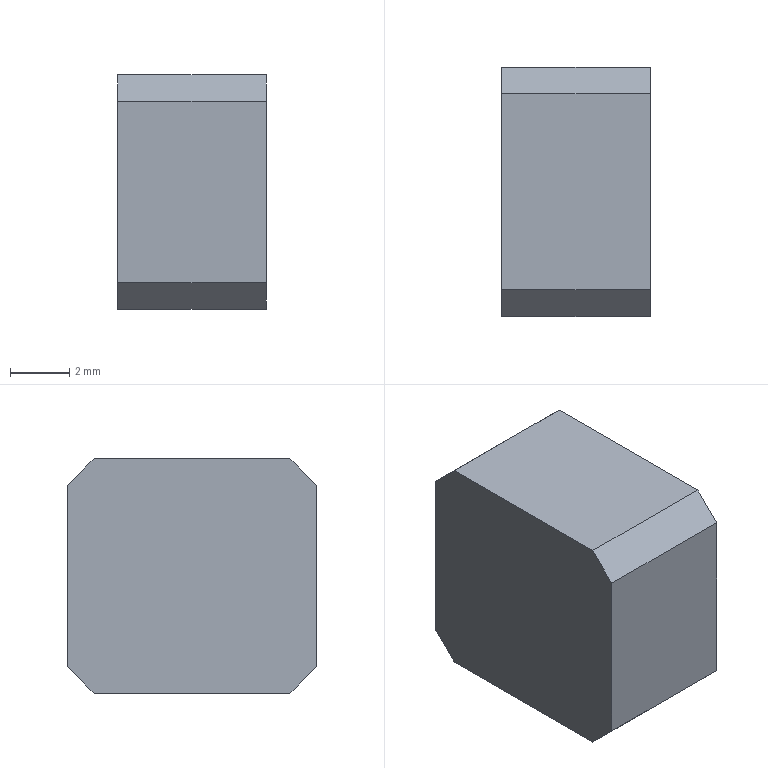Part | SolidWorks | features ICE 5, Chamfer 2, MoveFace 2, Extrusion 1 | 1 solid | 13 faces | box 5 x 8.4 x 7.9 mm | volume 224.151 mm3 | plane 11 | cylinder 2 | commonest cylinder face diameters 6.5 x2
STEP:
#1=CARTESIAN_POINT('',(0.,0.,3.25));
#2=VERTEX_POINT('',#1);
#3=CARTESIAN_POINT('',(0.,0.,-3.25));
#4=VERTEX_POINT('',#3);
#5=CARTESIAN_POINT('',(0.,0.,0.));
#6=DIRECTION('',(1.,0.,0.));
#7=DIRECTION('',(0.,0.,-1.));
#8=AXIS2_PLACEMENT_3D('',#5,#6,#7);
#9=CIRCLE('',#8,3.25);
#10=EDGE_CURVE('',#2,#4,#9,.T.);
#11=ORIENTED_EDGE('',*,*,#10,.F.);
#12=CARTESIAN_POINT('',(3.,0.,3.25));
#13=VERTEX_POINT('',#12);
#14=CARTESIAN_POINT('',(0.,0.,3.25));
#15=DIRECTION('',(1.,0.,0.));
#16=VECTOR('',#15,1000.);
#17=LINE('',#14,#16);
#18=EDGE_CURVE('',#2,#13,#17,.T.);
#19=ORIENTED_EDGE('',*,*,#18,.T.);
#20=CARTESIAN_POINT('',(3.,0.,-3.25));
#21=VERTEX_POINT('',#20);
#22=CARTESIAN_POINT('',(3.,0.,0.));
#23=DIRECTION('',(1.,0.,0.));
#24=DIRECTION('',(0.,0.,-1.));
#25=AXIS2_PLACEMENT_3D('',#22,#23,#24);
#26=CIRCLE('',#25,3.25);
#27=EDGE_CURVE('',#13,#21,#26,.T.);
#28=ORIENTED_EDGE('',*,*,#27,.T.);
#29=CARTESIAN_POINT('',(0.,0.,-3.25));
#30=DIRECTION('',(1.,0.,0.));
#31=VECTOR('',#30,1000.);
#32=LINE('',#29,#31);
#33=EDGE_CURVE('',#4,#21,#32,.T.);
#34=ORIENTED_EDGE('',*,*,#33,.F.);
#35=EDGE_LOOP('',(#11,#19,#28,#34));
#36=FACE_OUTER_BOUND('',#35,.T.);
#37=CARTESIAN_POINT('',(0.,0.,0.));
#38=DIRECTION('',(1.,0.,0.));
#39=DIRECTION('',(0.,0.,-1.));
#40=AXIS2_PLACEMENT_3D('',#37,#38,#39);
#41=CYLINDRICAL_SURFACE('',#40,3.25);
#42=ADVANCED_FACE('',(#36),#41,.F.);
#43=CARTESIAN_POINT('',(3.,3.3,3.95));
#44=VERTEX_POINT('',#43);
#45=CARTESIAN_POINT('',(3.,-3.3,3.95));
#46=VERTEX_POINT('',#45);
#47=CARTESIAN_POINT('',(3.,4.25,3.95));
#48=DIRECTION('',(0.,-1.,0.));
#49=VECTOR('',#48,1000.);
#50=LINE('',#47,#49);
#51=EDGE_CURVE('',#44,#46,#50,.T.);
#52=ORIENTED_EDGE('',*,*,#51,.F.);
#53=CARTESIAN_POINT('',(-2.,3.3,3.95));
#54=VERTEX_POINT('',#53);
#55=CARTESIAN_POINT('',(0.,3.3,3.95));
#56=DIRECTION('',(-1.,0.,0.));
#57=VECTOR('',#56,1000.);
#58=LINE('',#55,#57);
#59=EDGE_CURVE('',#44,#54,#58,.T.);
#60=ORIENTED_EDGE('',*,*,#59,.T.);
#61=CARTESIAN_POINT('',(-2.,-3.3,3.95));
#62=VERTEX_POINT('',#61);
#63=CARTESIAN_POINT('',(-2.,13.194,3.95));
#64=DIRECTION('',(0.,-1.,0.));
#65=VECTOR('',#64,1000.);
#66=LINE('',#63,#65);
#67=EDGE_CURVE('',#54,#62,#66,.T.);
#68=ORIENTED_EDGE('',*,*,#67,.T.);
#69=CARTESIAN_POINT('',(0.,-3.3,3.95));
#70=DIRECTION('',(1.,0.,0.));
#71=VECTOR('',#70,1000.);
#72=LINE('',#69,#71);
#73=EDGE_CURVE('',#62,#46,#72,.T.);
#74=ORIENTED_EDGE('',*,*,#73,.T.);
#75=EDGE_LOOP('',(#52,#60,#68,#74));
#76=FACE_OUTER_BOUND('',#75,.T.);
#77=CARTESIAN_POINT('',(0.,4.25,3.95));
#78=DIRECTION('',(0.,0.,-1.));
#79=DIRECTION('',(-1.,0.,0.));
#80=AXIS2_PLACEMENT_3D('',#77,#78,#79);
#81=PLANE('',#80);
#82=ADVANCED_FACE('',(#76),#81,.F.);
#83=CARTESIAN_POINT('',(3.,0.,0.));
#84=DIRECTION('',(1.,0.,0.));
#85=DIRECTION('',(0.,0.,-1.));
#86=AXIS2_PLACEMENT_3D('',#83,#84,#85);
#87=CIRCLE('',#86,3.25);
#88=EDGE_CURVE('',#21,#13,#87,.T.);
#89=ORIENTED_EDGE('',*,*,#88,.F.);
#90=ORIENTED_EDGE('',*,*,#27,.F.);
#91=EDGE_LOOP('',(#89,#90));
#92=FACE_BOUND('',#91,.T.);
#93=CARTESIAN_POINT('',(3.,3.3,-3.95));
#94=VERTEX_POINT('',#93);
#95=CARTESIAN_POINT('',(3.,-3.3,-3.95));
#96=VERTEX_POINT('',#95);
#97=CARTESIAN_POINT('',(3.,4.25,-3.95));
#98=DIRECTION('',(0.,-1.,0.));
#99=VECTOR('',#98,1000.);
#100=LINE('',#97,#99);
#101=EDGE_CURVE('',#94,#96,#100,.T.);
#102=ORIENTED_EDGE('',*,*,#101,.F.);
#103=CARTESIAN_POINT('',(3.,4.2,-3.05));
#104=VERTEX_POINT('',#103);
#105=CARTESIAN_POINT('',(3.,4.25,-3.));
#106=DIRECTION('',(0.,0.7071,0.7071));
#107=VECTOR('',#106,1000.);
#108=LINE('',#105,#107);
#109=EDGE_CURVE('',#94,#104,#108,.T.);
#110=ORIENTED_EDGE('',*,*,#109,.T.);
#111=CARTESIAN_POINT('',(3.,4.2,3.05));
#112=VERTEX_POINT('',#111);
#113=CARTESIAN_POINT('',(3.,4.2,-4.));
#114=DIRECTION('',(0.,0.,-1.));
#115=VECTOR('',#114,1000.);
#116=LINE('',#113,#115);
#117=EDGE_CURVE('',#112,#104,#116,.T.);
#118=ORIENTED_EDGE('',*,*,#117,.F.);
#119=CARTESIAN_POINT('',(3.,4.25,3.));
#120=DIRECTION('',(0.,-0.7071,0.7071));
#121=VECTOR('',#120,1000.);
#122=LINE('',#119,#121);
#123=EDGE_CURVE('',#112,#44,#122,.T.);
#124=ORIENTED_EDGE('',*,*,#123,.T.);
#125=ORIENTED_EDGE('',*,*,#51,.T.);
#126=CARTESIAN_POINT('',(3.,-4.2,3.05));
#127=VERTEX_POINT('',#126);
#128=CARTESIAN_POINT('',(3.,-3.25,4.));
#129=DIRECTION('',(0.,-0.7071,-0.7071));
#130=VECTOR('',#129,1000.);
#131=LINE('',#128,#130);
#132=EDGE_CURVE('',#46,#127,#131,.T.);
#133=ORIENTED_EDGE('',*,*,#132,.T.);
#134=CARTESIAN_POINT('',(3.,-4.2,-3.05));
#135=VERTEX_POINT('',#134);
#136=CARTESIAN_POINT('',(3.,-4.2,-4.));
#137=DIRECTION('',(0.,0.,-1.));
#138=VECTOR('',#137,1000.);
#139=LINE('',#136,#138);
#140=EDGE_CURVE('',#127,#135,#139,.T.);
#141=ORIENTED_EDGE('',*,*,#140,.T.);
#142=CARTESIAN_POINT('',(3.,-3.25,-4.));
#143=DIRECTION('',(0.,0.7071,-0.7071));
#144=VECTOR('',#143,1000.);
#145=LINE('',#142,#144);
#146=EDGE_CURVE('',#135,#96,#145,.T.);
#147=ORIENTED_EDGE('',*,*,#146,.T.);
#148=EDGE_LOOP('',(#102,#110,#118,#124,#125,#133,#141,#147));
#149=FACE_OUTER_BOUND('',#148,.T.);
#150=CARTESIAN_POINT('',(3.,4.25,-4.));
#151=DIRECTION('',(-1.,0.,0.));
#152=DIRECTION('',(0.,0.,1.));
#153=AXIS2_PLACEMENT_3D('',#150,#151,#152);
#154=PLANE('',#153);
#155=ADVANCED_FACE('',(#92,#149),#154,.F.);
#156=CARTESIAN_POINT('',(-2.,3.3,-3.95));
#157=VERTEX_POINT('',#156);
#158=CARTESIAN_POINT('',(-2.,-3.3,-3.95));
#159=VERTEX_POINT('',#158);
#160=CARTESIAN_POINT('',(-2.,4.25,-3.95));
#161=DIRECTION('',(0.,-1.,0.));
#162=VECTOR('',#161,1000.);
#163=LINE('',#160,#162);
#164=EDGE_CURVE('',#157,#159,#163,.T.);
#165=ORIENTED_EDGE('',*,*,#164,.F.);
#166=CARTESIAN_POINT('',(0.,3.3,-3.95));
#167=DIRECTION('',(1.,0.,0.));
#168=VECTOR('',#167,1000.);
#169=LINE('',#166,#168);
#170=EDGE_CURVE('',#157,#94,#169,.T.);
#171=ORIENTED_EDGE('',*,*,#170,.T.);
#172=ORIENTED_EDGE('',*,*,#101,.T.);
#173=CARTESIAN_POINT('',(0.,-3.3,-3.95));
#174=DIRECTION('',(-1.,0.,0.));
#175=VECTOR('',#174,1000.);
#176=LINE('',#173,#175);
#177=EDGE_CURVE('',#96,#159,#176,.T.);
#178=ORIENTED_EDGE('',*,*,#177,.T.);
#179=EDGE_LOOP('',(#165,#171,#172,#178));
#180=FACE_OUTER_BOUND('',#179,.T.);
#181=CARTESIAN_POINT('',(0.,4.25,-3.95));
#182=DIRECTION('',(0.,0.,1.));
#183=DIRECTION('',(1.,0.,0.));
#184=AXIS2_PLACEMENT_3D('',#181,#182,#183);
#185=PLANE('',#184);
#186=ADVANCED_FACE('',(#180),#185,.F.);
#187=ORIENTED_EDGE('',*,*,#117,.T.);
#188=CARTESIAN_POINT('',(-2.,4.2,-3.05));
#189=VERTEX_POINT('',#188);
#190=CARTESIAN_POINT('',(0.,4.2,-3.05));
#191=DIRECTION('',(-1.,0.,0.));
#192=VECTOR('',#191,1000.);
#193=LINE('',#190,#192);
#194=EDGE_CURVE('',#104,#189,#193,.T.);
#195=ORIENTED_EDGE('',*,*,#194,.T.);
#196=CARTESIAN_POINT('',(-2.,4.2,3.05));
#197=VERTEX_POINT('',#196);
#198=CARTESIAN_POINT('',(-2.,4.2,4.));
#199=DIRECTION('',(0.,0.,-1.));
#200=VECTOR('',#199,1000.);
#201=LINE('',#198,#200);
#202=EDGE_CURVE('',#197,#189,#201,.T.);
#203=ORIENTED_EDGE('',*,*,#202,.F.);
#204=CARTESIAN_POINT('',(0.,4.2,3.05));
#205=DIRECTION('',(1.,0.,0.));
#206=VECTOR('',#205,1000.);
#207=LINE('',#204,#206);
#208=EDGE_CURVE('',#197,#112,#207,.T.);
#209=ORIENTED_EDGE('',*,*,#208,.T.);
#210=EDGE_LOOP('',(#187,#195,#203,#209));
#211=FACE_OUTER_BOUND('',#210,.T.);
#212=CARTESIAN_POINT('',(0.,4.2,0.));
#213=DIRECTION('',(0.,1.,0.));
#214=DIRECTION('',(0.,0.,1.));
#215=AXIS2_PLACEMENT_3D('',#212,#213,#214);
#216=PLANE('',#215);
#217=ADVANCED_FACE('',(#211),#216,.T.);
#218=CARTESIAN_POINT('',(-2.,-4.2,3.05));
#219=VERTEX_POINT('',#218);
#220=CARTESIAN_POINT('',(-2.,-4.2,-3.05));
#221=VERTEX_POINT('',#220);
#222=CARTESIAN_POINT('',(-2.,-4.2,4.));
#223=DIRECTION('',(0.,0.,-1.));
#224=VECTOR('',#223,1000.);
#225=LINE('',#222,#224);
#226=EDGE_CURVE('',#219,#221,#225,.T.);
#227=ORIENTED_EDGE('',*,*,#226,.T.);
#228=CARTESIAN_POINT('',(0.,-4.2,-3.05));
#229=DIRECTION('',(1.,0.,0.));
#230=VECTOR('',#229,1000.);
#231=LINE('',#228,#230);
#232=EDGE_CURVE('',#221,#135,#231,.T.);
#233=ORIENTED_EDGE('',*,*,#232,.T.);
#234=ORIENTED_EDGE('',*,*,#140,.F.);
#235=CARTESIAN_POINT('',(0.,-4.2,3.05));
#236=DIRECTION('',(-1.,0.,0.));
#237=VECTOR('',#236,1000.);
#238=LINE('',#235,#237);
#239=EDGE_CURVE('',#127,#219,#238,.T.);
#240=ORIENTED_EDGE('',*,*,#239,.T.);
#241=EDGE_LOOP('',(#227,#233,#234,#240));
#242=FACE_OUTER_BOUND('',#241,.T.);
#243=CARTESIAN_POINT('',(0.,-4.2,0.));
#244=DIRECTION('',(0.,1.,0.));
#245=DIRECTION('',(0.,0.,1.));
#246=AXIS2_PLACEMENT_3D('',#243,#244,#245);
#247=PLANE('',#246);
#248=ADVANCED_FACE('',(#242),#247,.F.);
#249=ORIENTED_EDGE('',*,*,#18,.F.);
#250=CARTESIAN_POINT('',(0.,0.,0.));
#251=DIRECTION('',(1.,0.,0.));
#252=DIRECTION('',(0.,0.,-1.));
#253=AXIS2_PLACEMENT_3D('',#250,#251,#252);
#254=CIRCLE('',#253,3.25);
#255=EDGE_CURVE('',#4,#2,#254,.T.);
#256=ORIENTED_EDGE('',*,*,#255,.F.);
#257=ORIENTED_EDGE('',*,*,#33,.T.);
#258=ORIENTED_EDGE('',*,*,#88,.T.);
#259=EDGE_LOOP('',(#249,#256,#257,#258));
#260=FACE_OUTER_BOUND('',#259,.T.);
#261=CARTESIAN_POINT('',(0.,0.,0.));
#262=DIRECTION('',(1.,0.,0.));
#263=DIRECTION('',(0.,0.,-1.));
#264=AXIS2_PLACEMENT_3D('',#261,#262,#263);
#265=CYLINDRICAL_SURFACE('',#264,3.25);
#266=ADVANCED_FACE('',(#260),#265,.F.);
#267=ORIENTED_EDGE('',*,*,#255,.T.);
#268=ORIENTED_EDGE('',*,*,#10,.T.);
#269=EDGE_LOOP('',(#267,#268));
#270=FACE_OUTER_BOUND('',#269,.T.);
#271=CARTESIAN_POINT('',(0.,0.,0.));
#272=DIRECTION('',(1.,0.,0.));
#273=DIRECTION('',(0.,0.,-1.));
#274=AXIS2_PLACEMENT_3D('',#271,#272,#273);
#275=PLANE('',#274);
#276=ADVANCED_FACE('',(#270),#275,.T.);
#277=ORIENTED_EDGE('',*,*,#202,.T.);
#278=CARTESIAN_POINT('',(-2.,12.222,4.972));
#279=DIRECTION('',(0.,-0.7071,-0.7071));
#280=VECTOR('',#279,1000.);
#281=LINE('',#278,#280);
#282=EDGE_CURVE('',#189,#157,#281,.T.);
#283=ORIENTED_EDGE('',*,*,#282,.T.);
#284=ORIENTED_EDGE('',*,*,#164,.T.);
#285=CARTESIAN_POINT('',(-2.,0.9721,-8.222));
#286=DIRECTION('',(0.,-0.7071,0.7071));
#287=VECTOR('',#286,1000.);
#288=LINE('',#285,#287);
#289=EDGE_CURVE('',#159,#221,#288,.T.);
#290=ORIENTED_EDGE('',*,*,#289,.T.);
#291=ORIENTED_EDGE('',*,*,#226,.F.);
#292=CARTESIAN_POINT('',(-2.,4.972,12.222));
#293=DIRECTION('',(0.,0.7071,0.7071));
#294=VECTOR('',#293,1000.);
#295=LINE('',#292,#294);
#296=EDGE_CURVE('',#219,#62,#295,.T.);
#297=ORIENTED_EDGE('',*,*,#296,.T.);
#298=ORIENTED_EDGE('',*,*,#67,.F.);
#299=CARTESIAN_POINT('',(-2.,8.222,-0.9721));
#300=DIRECTION('',(0.,0.7071,-0.7071));
#301=VECTOR('',#300,1000.);
#302=LINE('',#299,#301);
#303=EDGE_CURVE('',#54,#197,#302,.T.);
#304=ORIENTED_EDGE('',*,*,#303,.T.);
#305=EDGE_LOOP('',(#277,#283,#284,#290,#291,#297,#298,#304));
#306=FACE_OUTER_BOUND('',#305,.T.);
#307=CARTESIAN_POINT('',(-2.,13.194,4.));
#308=DIRECTION('',(-1.,0.,0.));
#309=DIRECTION('',(0.,0.,1.));
#310=AXIS2_PLACEMENT_3D('',#307,#308,#309);
#311=PLANE('',#310);
#312=ADVANCED_FACE('',(#306),#311,.T.);
#313=ORIENTED_EDGE('',*,*,#109,.F.);
#314=ORIENTED_EDGE('',*,*,#170,.F.);
#315=ORIENTED_EDGE('',*,*,#282,.F.);
#316=ORIENTED_EDGE('',*,*,#194,.F.);
#317=EDGE_LOOP('',(#313,#314,#315,#316));
#318=FACE_OUTER_BOUND('',#317,.T.);
#319=CARTESIAN_POINT('',(0.,4.25,-3.));
#320=DIRECTION('',(0.,0.7071,-0.7071));
#321=DIRECTION('',(1.,0.,0.));
#322=AXIS2_PLACEMENT_3D('',#319,#320,#321);
#323=PLANE('',#322);
#324=ADVANCED_FACE('',(#318),#323,.T.);
#325=ORIENTED_EDGE('',*,*,#146,.F.);
#326=ORIENTED_EDGE('',*,*,#232,.F.);
#327=ORIENTED_EDGE('',*,*,#289,.F.);
#328=ORIENTED_EDGE('',*,*,#177,.F.);
#329=EDGE_LOOP('',(#325,#326,#327,#328));
#330=FACE_OUTER_BOUND('',#329,.T.);
#331=CARTESIAN_POINT('',(0.,-3.25,-4.));
#332=DIRECTION('',(0.,0.7071,0.7071));
#333=DIRECTION('',(-1.,0.,0.));
#334=AXIS2_PLACEMENT_3D('',#331,#332,#333);
#335=PLANE('',#334);
#336=ADVANCED_FACE('',(#330),#335,.F.);
#337=ORIENTED_EDGE('',*,*,#303,.F.);
#338=ORIENTED_EDGE('',*,*,#59,.F.);
#339=ORIENTED_EDGE('',*,*,#123,.F.);
#340=ORIENTED_EDGE('',*,*,#208,.F.);
#341=EDGE_LOOP('',(#337,#338,#339,#340));
#342=FACE_OUTER_BOUND('',#341,.T.);
#343=CARTESIAN_POINT('',(0.,4.25,3.));
#344=DIRECTION('',(0.,0.7071,0.7071));
#345=DIRECTION('',(-1.,0.,0.));
#346=AXIS2_PLACEMENT_3D('',#343,#344,#345);
#347=PLANE('',#346);
#348=ADVANCED_FACE('',(#342),#347,.T.);
#349=ORIENTED_EDGE('',*,*,#296,.F.);
#350=ORIENTED_EDGE('',*,*,#239,.F.);
#351=ORIENTED_EDGE('',*,*,#132,.F.);
#352=ORIENTED_EDGE('',*,*,#73,.F.);
#353=EDGE_LOOP('',(#349,#350,#351,#352));
#354=FACE_OUTER_BOUND('',#353,.T.);
#355=CARTESIAN_POINT('',(0.,-3.25,4.));
#356=DIRECTION('',(0.,0.7071,-0.7071));
#357=DIRECTION('',(1.,0.,0.));
#358=AXIS2_PLACEMENT_3D('',#355,#356,#357);
#359=PLANE('',#358);
#360=ADVANCED_FACE('',(#354),#359,.F.);
#361=CLOSED_SHELL('',(#42,#82,#155,#186,#217,#248,#266,#276,#312,#324,#336,#348,#360));
#362=MANIFOLD_SOLID_BREP('',#361);
#363=CARTESIAN_POINT('',(0.,0.,0.));
#364=DIRECTION('',(0.,0.,1.));
#365=DIRECTION('',(1.,0.,0.));
#366=AXIS2_PLACEMENT_3D('',#363,#364,#365);
#367=(LENGTH_UNIT()NAMED_UNIT(*)SI_UNIT(.MILLI.,.METRE.));
#368=UNCERTAINTY_MEASURE_WITH_UNIT(LENGTH_MEASURE(0.00001),#367,'','');
#369=(NAMED_UNIT(*)PLANE_ANGLE_UNIT()SI_UNIT($,.RADIAN.));
#370=(NAMED_UNIT(*)SI_UNIT($,.STERADIAN.)SOLID_ANGLE_UNIT());
#371=(GEOMETRIC_REPRESENTATION_CONTEXT(3)GLOBAL_UNCERTAINTY_ASSIGNED_CONTEXT((#368))GLOBAL_UNIT_ASSIGNED_CONTEXT((#367,#369,#370))REPRESENTATION_CONTEXT('',''));
#372=ADVANCED_BREP_SHAPE_REPRESENTATION('',(#362,#366),#371);